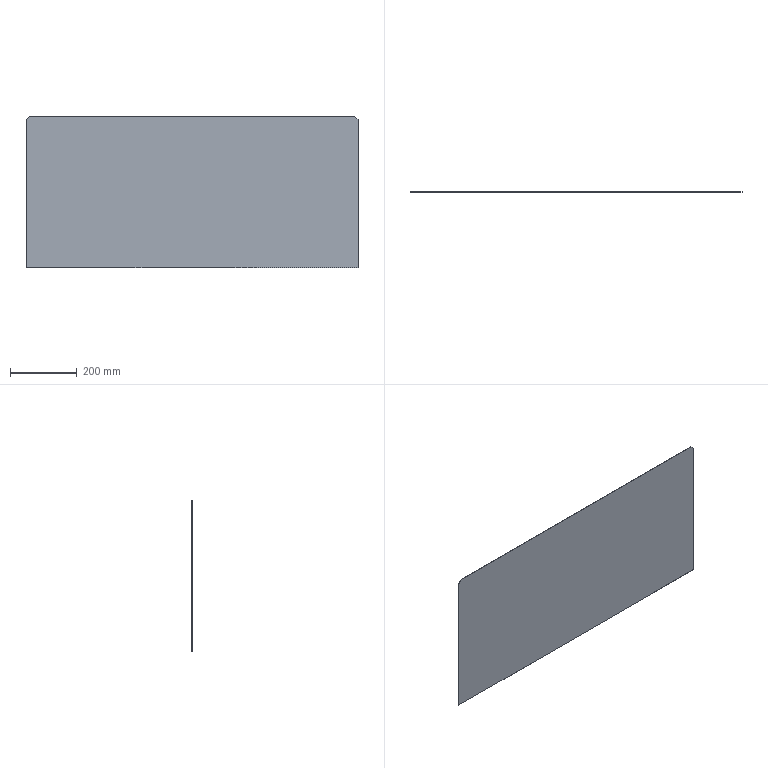Part | SolidWorks | features FlatPattern 1, SMBaseFlange 1, SheetMetal 1 | 1 solid | 8 faces | box 994.2 x 2.032 x 454.9 mm | volume 918733 mm3 | plane 8
STEP:
#1=CARTESIAN_POINT('',(52.074,102.8,45.653));
#2=VERTEX_POINT('',#1);
#3=CARTESIAN_POINT('',(-45.074,102.8,45.653));
#4=VERTEX_POINT('',#3);
#5=CARTESIAN_POINT('',(52.074,102.8,45.653));
#6=DIRECTION('',(-1.,0.,0.));
#7=VECTOR('',#6,100.);
#8=LINE('',#5,#7);
#9=EDGE_CURVE('',#2,#4,#8,.T.);
#10=ORIENTED_EDGE('',*,*,#9,.F.);
#11=CARTESIAN_POINT('',(52.074,103.003,45.653));
#12=VERTEX_POINT('',#11);
#13=CARTESIAN_POINT('',(52.074,103.003,45.653));
#14=DIRECTION('',(0.,-1.,0.));
#15=VECTOR('',#14,100.);
#16=LINE('',#13,#15);
#17=EDGE_CURVE('',#12,#2,#16,.T.);
#18=ORIENTED_EDGE('',*,*,#17,.F.);
#19=CARTESIAN_POINT('',(-45.074,103.003,45.653));
#20=VERTEX_POINT('',#19);
#21=CARTESIAN_POINT('',(52.074,103.003,45.653));
#22=DIRECTION('',(-1.,0.,0.));
#23=VECTOR('',#22,100.);
#24=LINE('',#21,#23);
#25=EDGE_CURVE('',#12,#20,#24,.T.);
#26=ORIENTED_EDGE('',*,*,#25,.T.);
#27=CARTESIAN_POINT('',(-45.074,103.003,45.653));
#28=DIRECTION('',(0.,-1.,0.));
#29=VECTOR('',#28,100.);
#30=LINE('',#27,#29);
#31=EDGE_CURVE('',#20,#4,#30,.T.);
#32=ORIENTED_EDGE('',*,*,#31,.T.);
#33=EDGE_LOOP('',(#10,#18,#26,#32));
#34=FACE_OUTER_BOUND('',#33,.T.);
#35=CARTESIAN_POINT('',(52.074,103.003,45.653));
#36=DIRECTION('',(0.,0.,1.));
#37=DIRECTION('',(0.,-1.,0.));
#38=AXIS2_PLACEMENT_3D('',#35,#36,#37);
#39=PLANE('',#38);
#40=ADVANCED_FACE('',(#34),#39,.T.);
#41=CARTESIAN_POINT('',(53.21,102.8,44.517));
#42=VERTEX_POINT('',#41);
#43=CARTESIAN_POINT('',(53.21,102.8,44.517));
#44=DIRECTION('',(-0.7071,0.,0.7071));
#45=VECTOR('',#44,100.);
#46=LINE('',#43,#45);
#47=EDGE_CURVE('',#42,#2,#46,.T.);
#48=ORIENTED_EDGE('',*,*,#47,.F.);
#49=CARTESIAN_POINT('',(53.21,103.003,44.517));
#50=VERTEX_POINT('',#49);
#51=CARTESIAN_POINT('',(53.21,103.003,44.517));
#52=DIRECTION('',(0.,-1.,0.));
#53=VECTOR('',#52,100.);
#54=LINE('',#51,#53);
#55=EDGE_CURVE('',#50,#42,#54,.T.);
#56=ORIENTED_EDGE('',*,*,#55,.F.);
#57=CARTESIAN_POINT('',(53.21,103.003,44.517));
#58=DIRECTION('',(-0.7071,0.,0.7071));
#59=VECTOR('',#58,100.);
#60=LINE('',#57,#59);
#61=EDGE_CURVE('',#50,#12,#60,.T.);
#62=ORIENTED_EDGE('',*,*,#61,.T.);
#63=ORIENTED_EDGE('',*,*,#17,.T.);
#64=EDGE_LOOP('',(#48,#56,#62,#63));
#65=FACE_OUTER_BOUND('',#64,.T.);
#66=CARTESIAN_POINT('',(53.21,103.003,44.517));
#67=DIRECTION('',(0.7071,0.,0.7071));
#68=DIRECTION('',(0.7071,0.,-0.7071));
#69=AXIS2_PLACEMENT_3D('',#66,#67,#68);
#70=PLANE('',#69);
#71=ADVANCED_FACE('',(#65),#70,.T.);
#72=CARTESIAN_POINT('',(53.21,102.8,0.1632));
#73=VERTEX_POINT('',#72);
#74=CARTESIAN_POINT('',(53.21,102.8,0.1632));
#75=DIRECTION('',(0.,0.,1.));
#76=VECTOR('',#75,100.);
#77=LINE('',#74,#76);
#78=EDGE_CURVE('',#73,#42,#77,.T.);
#79=ORIENTED_EDGE('',*,*,#78,.F.);
#80=CARTESIAN_POINT('',(53.21,103.003,0.1632));
#81=VERTEX_POINT('',#80);
#82=CARTESIAN_POINT('',(53.21,103.003,0.1632));
#83=DIRECTION('',(0.,-1.,0.));
#84=VECTOR('',#83,100.);
#85=LINE('',#82,#84);
#86=EDGE_CURVE('',#81,#73,#85,.T.);
#87=ORIENTED_EDGE('',*,*,#86,.F.);
#88=CARTESIAN_POINT('',(53.21,103.003,0.1632));
#89=DIRECTION('',(0.,0.,1.));
#90=VECTOR('',#89,100.);
#91=LINE('',#88,#90);
#92=EDGE_CURVE('',#81,#50,#91,.T.);
#93=ORIENTED_EDGE('',*,*,#92,.T.);
#94=ORIENTED_EDGE('',*,*,#55,.T.);
#95=EDGE_LOOP('',(#79,#87,#93,#94));
#96=FACE_OUTER_BOUND('',#95,.T.);
#97=CARTESIAN_POINT('',(53.21,103.003,0.1632));
#98=DIRECTION('',(1.,0.,0.));
#99=DIRECTION('',(0.,0.,-1.));
#100=AXIS2_PLACEMENT_3D('',#97,#98,#99);
#101=PLANE('',#100);
#102=ADVANCED_FACE('',(#96),#101,.T.);
#103=CARTESIAN_POINT('',(-46.21,102.8,0.1632));
#104=VERTEX_POINT('',#103);
#105=CARTESIAN_POINT('',(-46.21,102.8,0.1632));
#106=DIRECTION('',(1.,0.,0.));
#107=VECTOR('',#106,100.);
#108=LINE('',#105,#107);
#109=EDGE_CURVE('',#104,#73,#108,.T.);
#110=ORIENTED_EDGE('',*,*,#109,.F.);
#111=CARTESIAN_POINT('',(-46.21,103.003,0.1632));
#112=VERTEX_POINT('',#111);
#113=CARTESIAN_POINT('',(-46.21,103.003,0.1632));
#114=DIRECTION('',(0.,-1.,0.));
#115=VECTOR('',#114,100.);
#116=LINE('',#113,#115);
#117=EDGE_CURVE('',#112,#104,#116,.T.);
#118=ORIENTED_EDGE('',*,*,#117,.F.);
#119=CARTESIAN_POINT('',(-46.21,103.003,0.1632));
#120=DIRECTION('',(1.,0.,0.));
#121=VECTOR('',#120,100.);
#122=LINE('',#119,#121);
#123=EDGE_CURVE('',#112,#81,#122,.T.);
#124=ORIENTED_EDGE('',*,*,#123,.T.);
#125=ORIENTED_EDGE('',*,*,#86,.T.);
#126=EDGE_LOOP('',(#110,#118,#124,#125));
#127=FACE_OUTER_BOUND('',#126,.T.);
#128=CARTESIAN_POINT('',(-46.21,103.003,0.1632));
#129=DIRECTION('',(0.,0.,-1.));
#130=DIRECTION('',(0.,1.,0.));
#131=AXIS2_PLACEMENT_3D('',#128,#129,#130);
#132=PLANE('',#131);
#133=ADVANCED_FACE('',(#127),#132,.T.);
#134=CARTESIAN_POINT('',(-46.21,102.8,44.517));
#135=VERTEX_POINT('',#134);
#136=CARTESIAN_POINT('',(-46.21,102.8,44.517));
#137=DIRECTION('',(0.,0.,-1.));
#138=VECTOR('',#137,100.);
#139=LINE('',#136,#138);
#140=EDGE_CURVE('',#135,#104,#139,.T.);
#141=ORIENTED_EDGE('',*,*,#140,.F.);
#142=CARTESIAN_POINT('',(-46.21,103.003,44.517));
#143=VERTEX_POINT('',#142);
#144=CARTESIAN_POINT('',(-46.21,103.003,44.517));
#145=DIRECTION('',(0.,-1.,0.));
#146=VECTOR('',#145,100.);
#147=LINE('',#144,#146);
#148=EDGE_CURVE('',#143,#135,#147,.T.);
#149=ORIENTED_EDGE('',*,*,#148,.F.);
#150=CARTESIAN_POINT('',(-46.21,103.003,44.517));
#151=DIRECTION('',(0.,0.,-1.));
#152=VECTOR('',#151,100.);
#153=LINE('',#150,#152);
#154=EDGE_CURVE('',#143,#112,#153,.T.);
#155=ORIENTED_EDGE('',*,*,#154,.T.);
#156=ORIENTED_EDGE('',*,*,#117,.T.);
#157=EDGE_LOOP('',(#141,#149,#155,#156));
#158=FACE_OUTER_BOUND('',#157,.T.);
#159=CARTESIAN_POINT('',(-46.21,103.003,44.517));
#160=DIRECTION('',(-1.,0.,0.));
#161=DIRECTION('',(0.,0.,1.));
#162=AXIS2_PLACEMENT_3D('',#159,#160,#161);
#163=PLANE('',#162);
#164=ADVANCED_FACE('',(#158),#163,.T.);
#165=CARTESIAN_POINT('',(-45.074,102.8,45.653));
#166=DIRECTION('',(-0.7071,0.,-0.7071));
#167=VECTOR('',#166,100.);
#168=LINE('',#165,#167);
#169=EDGE_CURVE('',#4,#135,#168,.T.);
#170=ORIENTED_EDGE('',*,*,#169,.F.);
#171=ORIENTED_EDGE('',*,*,#31,.F.);
#172=CARTESIAN_POINT('',(-45.074,103.003,45.653));
#173=DIRECTION('',(-0.7071,0.,-0.7071));
#174=VECTOR('',#173,100.);
#175=LINE('',#172,#174);
#176=EDGE_CURVE('',#20,#143,#175,.T.);
#177=ORIENTED_EDGE('',*,*,#176,.T.);
#178=ORIENTED_EDGE('',*,*,#148,.T.);
#179=EDGE_LOOP('',(#170,#171,#177,#178));
#180=FACE_OUTER_BOUND('',#179,.T.);
#181=CARTESIAN_POINT('',(-45.074,103.003,45.653));
#182=DIRECTION('',(-0.7071,0.,0.7071));
#183=DIRECTION('',(0.7071,0.,0.7071));
#184=AXIS2_PLACEMENT_3D('',#181,#182,#183);
#185=PLANE('',#184);
#186=ADVANCED_FACE('',(#180),#185,.T.);
#187=ORIENTED_EDGE('',*,*,#25,.F.);
#188=ORIENTED_EDGE('',*,*,#61,.F.);
#189=ORIENTED_EDGE('',*,*,#92,.F.);
#190=ORIENTED_EDGE('',*,*,#123,.F.);
#191=ORIENTED_EDGE('',*,*,#154,.F.);
#192=ORIENTED_EDGE('',*,*,#176,.F.);
#193=EDGE_LOOP('',(#187,#188,#189,#190,#191,#192));
#194=FACE_OUTER_BOUND('',#193,.T.);
#195=CARTESIAN_POINT('',(0.,103.003,0.));
#196=DIRECTION('',(0.,-1.,0.));
#197=DIRECTION('',(0.,0.,-1.));
#198=AXIS2_PLACEMENT_3D('',#195,#196,#197);
#199=PLANE('',#198);
#200=ADVANCED_FACE('',(#194),#199,.F.);
#201=ORIENTED_EDGE('',*,*,#9,.T.);
#202=ORIENTED_EDGE('',*,*,#169,.T.);
#203=ORIENTED_EDGE('',*,*,#140,.T.);
#204=ORIENTED_EDGE('',*,*,#109,.T.);
#205=ORIENTED_EDGE('',*,*,#78,.T.);
#206=ORIENTED_EDGE('',*,*,#47,.T.);
#207=EDGE_LOOP('',(#201,#202,#203,#204,#205,#206));
#208=FACE_OUTER_BOUND('',#207,.T.);
#209=CARTESIAN_POINT('',(0.,102.8,0.));
#210=DIRECTION('',(0.,-1.,0.));
#211=DIRECTION('',(0.,0.,-1.));
#212=AXIS2_PLACEMENT_3D('',#209,#210,#211);
#213=PLANE('',#212);
#214=ADVANCED_FACE('',(#208),#213,.T.);
#215=CLOSED_SHELL('',(#40,#71,#102,#133,#164,#186,#200,#214));
#216=MANIFOLD_SOLID_BREP('',#215);
#217=CARTESIAN_POINT('',(0.,0.,0.));
#218=DIRECTION('',(0.,0.,1.));
#219=DIRECTION('',(1.,0.,0.));
#220=AXIS2_PLACEMENT_3D('',#217,#218,#219);
#221=(LENGTH_UNIT()NAMED_UNIT(*)SI_UNIT(.CENTI.,.METRE.));
#222=UNCERTAINTY_MEASURE_WITH_UNIT(LENGTH_MEASURE(0.00001),#221,'','');
#223=(NAMED_UNIT(*)PLANE_ANGLE_UNIT()SI_UNIT($,.RADIAN.));
#224=(NAMED_UNIT(*)SI_UNIT($,.STERADIAN.)SOLID_ANGLE_UNIT());
#225=(GEOMETRIC_REPRESENTATION_CONTEXT(3)GLOBAL_UNCERTAINTY_ASSIGNED_CONTEXT((#222))GLOBAL_UNIT_ASSIGNED_CONTEXT((#221,#223,#224))REPRESENTATION_CONTEXT('',''));
#226=ADVANCED_BREP_SHAPE_REPRESENTATION('',(#216,#220),#225);